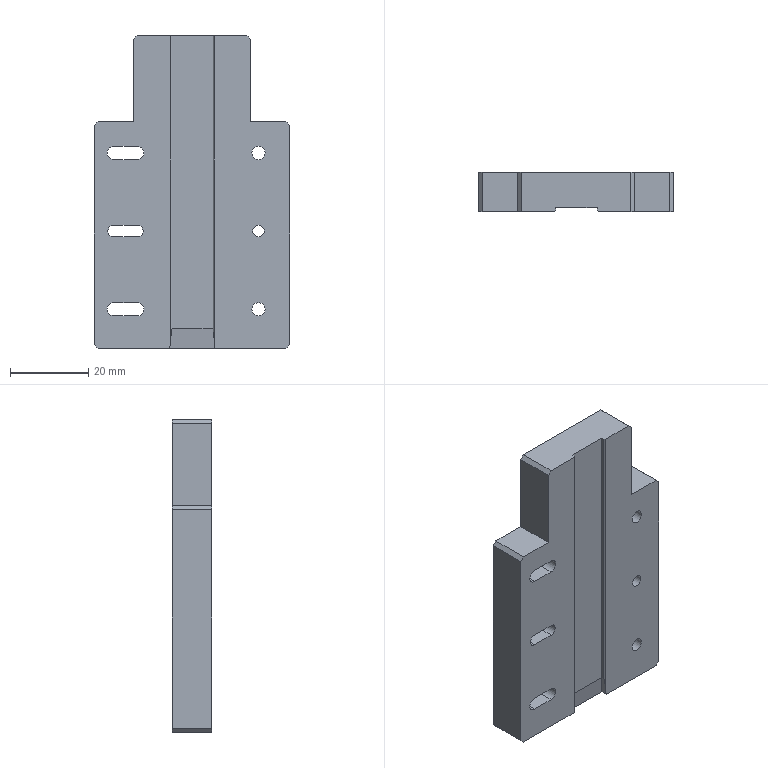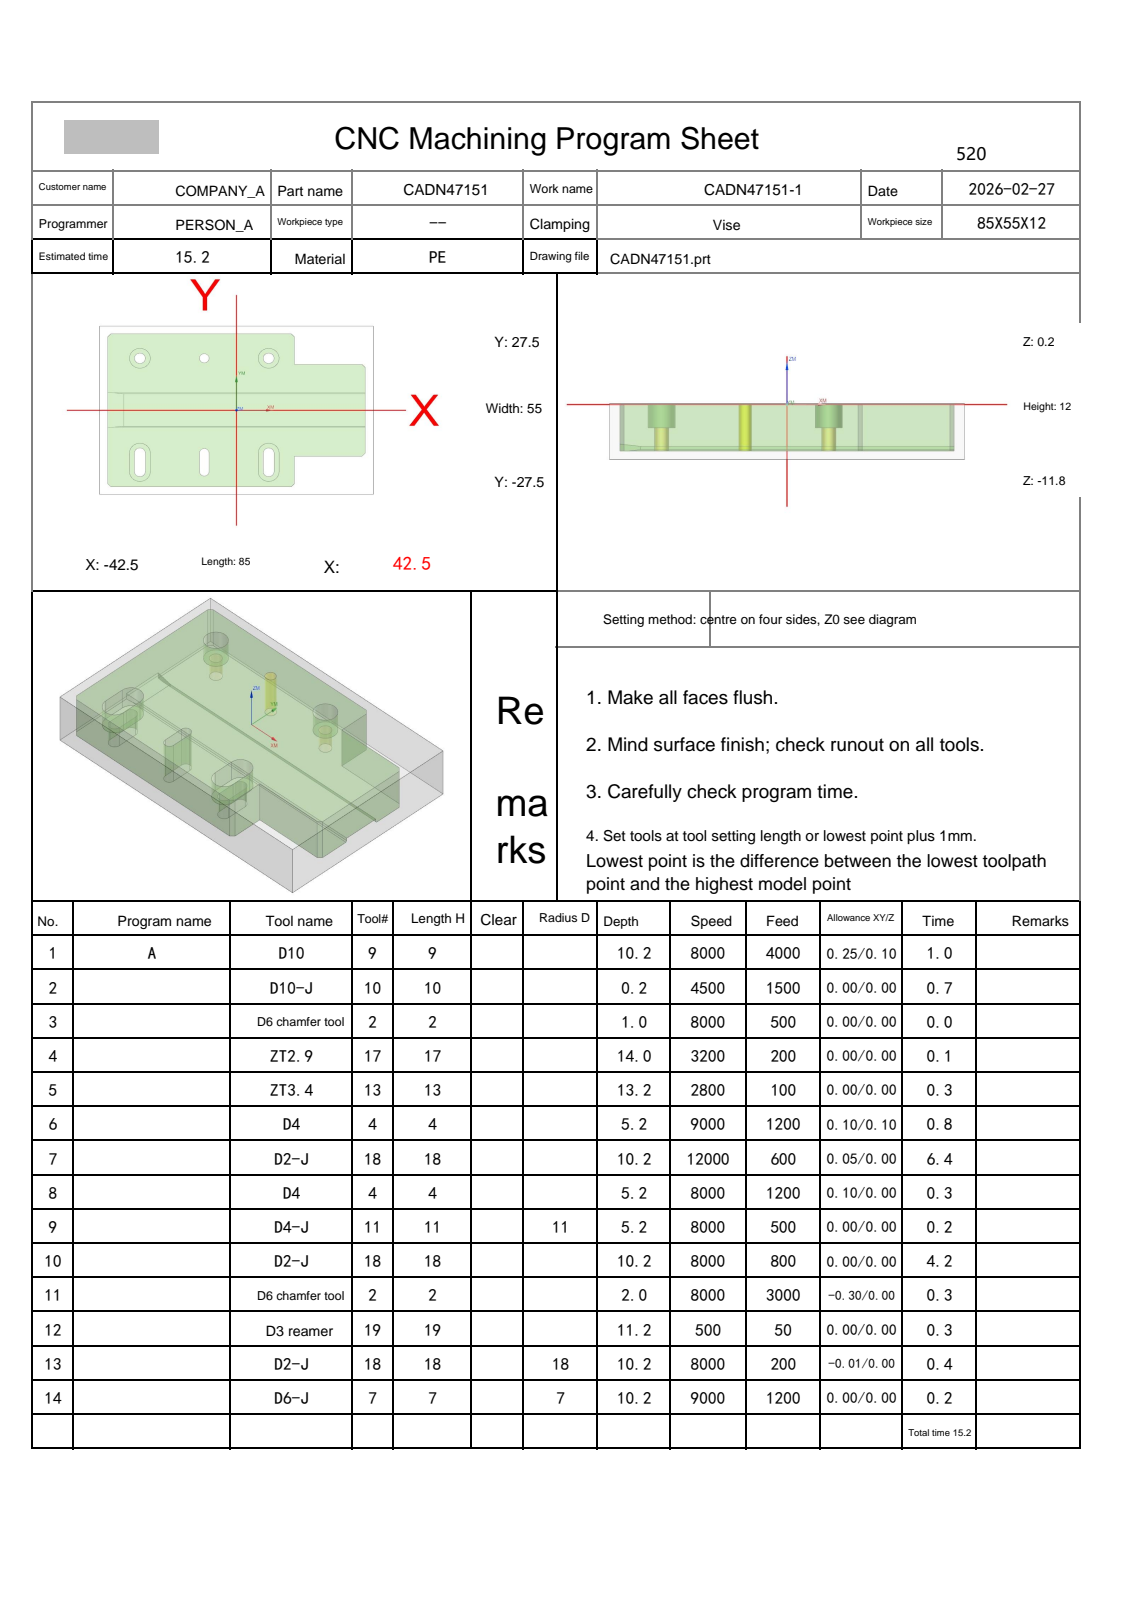NC program | NX | posted by the shop | part box 50 x 10 x 80 mm
Lines 2935 to 4061 of 8100:
N10 T18 M06
(D2-J  D=2. R=0. H=18 ce=0.00 di=0.00)
G00 G90 G54 X19.201 Y20.15 M03 S8000
G43 H18 Z50.
M08
Z.1
G01 X19.199 Y20.149 Z.07 F800.
X19.191 Y20.147 Z.042
X19.18 Y20.144 Z.018
X19.166 Y20.139 Z-.004
X19.149 Y20.133 Z-.023
X19.13 Y20.125 Z-.04
X19.111 Y20.115 Z-.054
X19.091 Y20.103 Z-.066
X19.071 Y20.089 Z-.076
X19.052 Y20.072 Z-.084
X19.035 Y20.053 Z-.09
X19.021 Y20.032 Z-.095
X19.01 Y20.007 Z-.098
X19.003 Y19.98 Z-.099
X19. Y19.95 Z-.1
Y16.
X22.95
X22.964 Y16.014
X22.953 Y16.056 Z-.101
X22.919 Y16.121 Z-.103
X22.864 Y16.209 Z-.104
X22.599 Y16.565 Z-.112
X22.346 Y16.878 Z-.119
X22.146 Y17.111 Z-.125
X21.909 Y17.375 Z-.131
X21.632 Y17.674 Z-.138
X21.322 Y17.995 Z-.146
X20.996 Y18.322 Z-.154
X20.674 Y18.632 Z-.162
X20.376 Y18.909 Z-.169
X20.111 Y19.146 Z-.175
X19.878 Y19.345 Z-.181
X19.566 Y19.599 Z-.188
X19.209 Y19.864 Z-.196
X19.121 Y19.919 Z-.197
X19.056 Y19.953 Z-.199
X19.014 Y19.964 Z-.2
X19. Y19.95
Y16.
X22.95
X22.964 Y16.014
X22.953 Y16.056 Z-.201
X22.919 Y16.121 Z-.203
X22.864 Y16.209 Z-.204
X22.599 Y16.565 Z-.212
X22.346 Y16.878 Z-.219
X22.146 Y17.111 Z-.225
X21.909 Y17.375 Z-.231
X21.632 Y17.674 Z-.238
X21.322 Y17.995 Z-.246
X20.996 Y18.322 Z-.254
X20.674 Y18.632 Z-.262
X20.376 Y18.909 Z-.269
X20.111 Y19.146 Z-.275
X19.878 Y19.345 Z-.281
X19.566 Y19.599 Z-.288
X19.209 Y19.864 Z-.296
X19.121 Y19.919 Z-.297
X19.056 Y19.953 Z-.299
X19.014 Y19.964 Z-.3
X19. Y19.95
Y16.
X22.95
X22.964 Y16.014
X22.953 Y16.056 Z-.301
X22.919 Y16.121 Z-.303
X22.864 Y16.209 Z-.304
X22.599 Y16.565 Z-.312
X22.346 Y16.878 Z-.319
X22.146 Y17.111 Z-.325
X21.909 Y17.375 Z-.331
X21.632 Y17.674 Z-.338
X21.322 Y17.995 Z-.346
X20.996 Y18.322 Z-.354
X20.674 Y18.632 Z-.362
X20.376 Y18.909 Z-.369
X20.111 Y19.146 Z-.375
X19.878 Y19.345 Z-.381
X19.566 Y19.599 Z-.388
X19.209 Y19.864 Z-.396
X19.121 Y19.919 Z-.397
X19.056 Y19.953 Z-.399
X19.014 Y19.964 Z-.4
X19. Y19.95
Y16.
X22.95
X22.964 Y16.014
X22.953 Y16.056 Z-.401
X22.919 Y16.121 Z-.403
X22.864 Y16.209 Z-.404
X22.599 Y16.565 Z-.412
X22.346 Y16.878 Z-.419
X22.146 Y17.111 Z-.425
X21.909 Y17.375 Z-.431
X21.632 Y17.674 Z-.438
X21.322 Y17.995 Z-.446
X20.996 Y18.322 Z-.454
X20.674 Y18.632 Z-.462
X20.376 Y18.909 Z-.469
X20.111 Y19.146 Z-.475
X19.878 Y19.345 Z-.481
X19.566 Y19.599 Z-.488
X19.209 Y19.864 Z-.496
X19.121 Y19.919 Z-.497
X19.056 Y19.953 Z-.499
X19.014 Y19.964 Z-.5
X19. Y19.95
Y16.
X22.95
X22.964 Y16.014
X22.953 Y16.056 Z-.501
X22.919 Y16.121 Z-.503
X22.864 Y16.209 Z-.504
X22.599 Y16.565 Z-.512
X22.346 Y16.878 Z-.519
X22.146 Y17.111 Z-.525
X21.909 Y17.375 Z-.531
X21.632 Y17.674 Z-.538
X21.322 Y17.995 Z-.546
X20.996 Y18.322 Z-.554
X20.674 Y18.632 Z-.562
X20.376 Y18.909 Z-.569
X20.111 Y19.146 Z-.575
X19.878 Y19.345 Z-.581
X19.566 Y19.599 Z-.588
X19.209 Y19.864 Z-.596
X19.121 Y19.919 Z-.597
X19.056 Y19.953 Z-.599
X19.014 Y19.964 Z-.6
X19. Y19.95
Y16.
X22.95
X22.964 Y16.014
X22.953 Y16.056 Z-.601
X22.919 Y16.121 Z-.603
X22.864 Y16.209 Z-.604
X22.599 Y16.565 Z-.612
X22.346 Y16.878 Z-.619
X22.146 Y17.111 Z-.625
X21.909 Y17.375 Z-.631
X21.632 Y17.674 Z-.638
X21.322 Y17.995 Z-.646
X20.996 Y18.322 Z-.654
X20.674 Y18.632 Z-.662
X20.376 Y18.909 Z-.669
X20.111 Y19.146 Z-.675
X19.878 Y19.345 Z-.681
X19.566 Y19.599 Z-.688
X19.209 Y19.864 Z-.696
X19.121 Y19.919 Z-.697
X19.056 Y19.953 Z-.699
X19.014 Y19.964 Z-.7
X19. Y19.95
Y16.
X22.95
X22.964 Y16.014
X22.953 Y16.056 Z-.701
X22.919 Y16.121 Z-.703
X22.864 Y16.209 Z-.704
X22.599 Y16.565 Z-.712
X22.346 Y16.878 Z-.719
X22.146 Y17.111 Z-.725
X21.909 Y17.375 Z-.731
X21.632 Y17.674 Z-.738
X21.322 Y17.995 Z-.746
X20.996 Y18.322 Z-.754
X20.674 Y18.632 Z-.762
X20.376 Y18.909 Z-.769
X20.111 Y19.146 Z-.775
X19.878 Y19.345 Z-.781
X19.566 Y19.599 Z-.788
X19.209 Y19.864 Z-.796
X19.121 Y19.919 Z-.797
X19.056 Y19.953 Z-.799
X19.014 Y19.964 Z-.8
X19. Y19.95
Y16.
X22.95
X22.964 Y16.014
X22.953 Y16.056 Z-.801
X22.919 Y16.121 Z-.803
X22.864 Y16.209 Z-.804
X22.599 Y16.565 Z-.812
X22.346 Y16.878 Z-.819
X22.146 Y17.111 Z-.825
X21.909 Y17.375 Z-.831
X21.632 Y17.674 Z-.838
X21.322 Y17.995 Z-.846
X20.996 Y18.322 Z-.854
X20.674 Y18.632 Z-.862
X20.376 Y18.909 Z-.869
X20.111 Y19.146 Z-.875
X19.878 Y19.345 Z-.881
X19.566 Y19.599 Z-.888
X19.209 Y19.864 Z-.896
X19.121 Y19.919 Z-.897
X19.056 Y19.953 Z-.899
X19.014 Y19.964 Z-.9
X19. Y19.95
Y16.
X22.95
X22.964 Y16.014
X22.953 Y16.056 Z-.901
X22.919 Y16.121 Z-.903
X22.864 Y16.209 Z-.904
X22.599 Y16.565 Z-.912
X22.346 Y16.878 Z-.919
X22.146 Y17.111 Z-.925
X21.909 Y17.375 Z-.931
X21.632 Y17.674 Z-.938
X21.322 Y17.995 Z-.946
X20.996 Y18.322 Z-.954
X20.674 Y18.632 Z-.962
X20.376 Y18.909 Z-.969
X20.111 Y19.146 Z-.975
X19.878 Y19.345 Z-.981
X19.566 Y19.599 Z-.988
X19.209 Y19.864 Z-.996
X19.121 Y19.919 Z-.997
X19.056 Y19.953 Z-.999
X19.014 Y19.964 Z-1.
X19. Y19.95
Y16.
X22.95
X22.964 Y16.014
X22.953 Y16.056 Z-1.001
X22.919 Y16.121 Z-1.003
X22.864 Y16.209 Z-1.004
X22.599 Y16.565 Z-1.012
X22.346 Y16.878 Z-1.019
X22.146 Y17.111 Z-1.025
X21.909 Y17.375 Z-1.031
X21.632 Y17.674 Z-1.038
X21.322 Y17.995 Z-1.046
X20.996 Y18.322 Z-1.054
X20.674 Y18.632 Z-1.062
X20.376 Y18.909 Z-1.069
X20.111 Y19.146 Z-1.075
X19.878 Y19.345 Z-1.081
X19.566 Y19.599 Z-1.088
X19.209 Y19.864 Z-1.096
X19.121 Y19.919 Z-1.097
X19.056 Y19.953 Z-1.099
X19.014 Y19.964 Z-1.1
X19. Y19.95
Y16.
X22.95
X22.964 Y16.014
X22.953 Y16.056 Z-1.101
X22.919 Y16.121 Z-1.103
X22.864 Y16.209 Z-1.104
X22.599 Y16.565 Z-1.112
X22.346 Y16.878 Z-1.119
X22.146 Y17.111 Z-1.125
X21.909 Y17.375 Z-1.131
X21.632 Y17.674 Z-1.138
X21.322 Y17.995 Z-1.146
X20.996 Y18.322 Z-1.154
X20.674 Y18.632 Z-1.162
X20.376 Y18.909 Z-1.169
X20.111 Y19.146 Z-1.175
X19.878 Y19.345 Z-1.181
X19.566 Y19.599 Z-1.188
X19.209 Y19.864 Z-1.196
X19.121 Y19.919 Z-1.197
X19.056 Y19.953 Z-1.199
X19.014 Y19.964 Z-1.2
X19. Y19.95
Y16.
X22.95
X22.964 Y16.014
X22.953 Y16.056 Z-1.201
X22.919 Y16.121 Z-1.203
X22.864 Y16.209 Z-1.204
X22.599 Y16.565 Z-1.212
X22.346 Y16.878 Z-1.219
X22.146 Y17.111 Z-1.225
X21.909 Y17.375 Z-1.231
X21.632 Y17.674 Z-1.238
X21.322 Y17.995 Z-1.246
X20.996 Y18.322 Z-1.254
X20.674 Y18.632 Z-1.262
X20.376 Y18.909 Z-1.269
X20.111 Y19.146 Z-1.275
X19.878 Y19.345 Z-1.281
X19.566 Y19.599 Z-1.288
X19.209 Y19.864 Z-1.296
X19.121 Y19.919 Z-1.297
X19.056 Y19.953 Z-1.299
X19.014 Y19.964 Z-1.3
X19. Y19.95
Y16.
X22.95
X22.964 Y16.014
X22.953 Y16.056 Z-1.301
X22.919 Y16.121 Z-1.303
X22.864 Y16.209 Z-1.304
X22.599 Y16.565 Z-1.312
X22.346 Y16.878 Z-1.319
X22.146 Y17.111 Z-1.325
X21.909 Y17.375 Z-1.331
X21.632 Y17.674 Z-1.338
X21.322 Y17.995 Z-1.346
X20.996 Y18.322 Z-1.354
X20.674 Y18.632 Z-1.362
X20.376 Y18.909 Z-1.369
X20.111 Y19.146 Z-1.375
X19.878 Y19.345 Z-1.381
X19.566 Y19.599 Z-1.388
X19.209 Y19.864 Z-1.396
X19.121 Y19.919 Z-1.397
X19.056 Y19.953 Z-1.399
X19.014 Y19.964 Z-1.4
X19. Y19.95
Y16.
X22.95
X22.964 Y16.014
X22.953 Y16.056 Z-1.401
X22.919 Y16.121 Z-1.403
X22.864 Y16.209 Z-1.404
X22.599 Y16.565 Z-1.412
X22.346 Y16.878 Z-1.419
X22.146 Y17.111 Z-1.425
X21.909 Y17.375 Z-1.431
X21.632 Y17.674 Z-1.438
X21.322 Y17.995 Z-1.446
X20.996 Y18.322 Z-1.454
X20.674 Y18.632 Z-1.462
X20.376 Y18.909 Z-1.469
X20.111 Y19.146 Z-1.475
X19.878 Y19.345 Z-1.481
X19.566 Y19.599 Z-1.488
X19.209 Y19.864 Z-1.496
X19.121 Y19.919 Z-1.497
X19.056 Y19.953 Z-1.499
X19.014 Y19.964 Z-1.5
X19. Y19.95
Y16.
X22.95
X22.964 Y16.014
X22.953 Y16.056 Z-1.501
X22.919 Y16.121 Z-1.503
X22.864 Y16.209 Z-1.504
X22.599 Y16.565 Z-1.512
X22.346 Y16.878 Z-1.519
X22.146 Y17.111 Z-1.525
X21.909 Y17.375 Z-1.531
X21.632 Y17.674 Z-1.538
X21.322 Y17.995 Z-1.546
X20.996 Y18.322 Z-1.554
X20.674 Y18.632 Z-1.562
X20.376 Y18.909 Z-1.569
X20.111 Y19.146 Z-1.575
X19.878 Y19.345 Z-1.581
X19.566 Y19.599 Z-1.588
X19.209 Y19.864 Z-1.596
X19.121 Y19.919 Z-1.597
X19.056 Y19.953 Z-1.599
X19.014 Y19.964 Z-1.6
X19. Y19.95
Y16.
X22.95
X22.964 Y16.014
X22.953 Y16.056 Z-1.601
X22.919 Y16.121 Z-1.603
X22.864 Y16.209 Z-1.604
X22.599 Y16.565 Z-1.612
X22.346 Y16.878 Z-1.619
X22.146 Y17.111 Z-1.625
X21.909 Y17.375 Z-1.631
X21.632 Y17.674 Z-1.638
X21.322 Y17.995 Z-1.646
X20.996 Y18.322 Z-1.654
X20.674 Y18.632 Z-1.662
X20.376 Y18.909 Z-1.669
X20.111 Y19.146 Z-1.675
X19.878 Y19.345 Z-1.681
X19.566 Y19.599 Z-1.688
X19.209 Y19.864 Z-1.696
X19.121 Y19.919 Z-1.697
X19.056 Y19.953 Z-1.699
X19.014 Y19.964 Z-1.7
X19. Y19.95
Y16.
X22.95
X22.964 Y16.014
X22.953 Y16.056 Z-1.701
X22.919 Y16.121 Z-1.703
X22.864 Y16.209 Z-1.704
X22.599 Y16.565 Z-1.712
X22.346 Y16.878 Z-1.719
X22.146 Y17.111 Z-1.725
X21.909 Y17.375 Z-1.731
X21.632 Y17.674 Z-1.738
X21.322 Y17.995 Z-1.746
X20.996 Y18.322 Z-1.754
X20.674 Y18.632 Z-1.762
X20.376 Y18.909 Z-1.769
X20.111 Y19.146 Z-1.775
X19.878 Y19.345 Z-1.781
X19.566 Y19.599 Z-1.788
X19.209 Y19.864 Z-1.796
X19.121 Y19.919 Z-1.797
X19.056 Y19.953 Z-1.799
X19.014 Y19.964 Z-1.8
X19. Y19.95
Y16.
X22.95
X22.964 Y16.014
X22.953 Y16.056 Z-1.801
X22.919 Y16.121 Z-1.803
X22.864 Y16.209 Z-1.804
X22.599 Y16.565 Z-1.812
X22.346 Y16.878 Z-1.819
X22.146 Y17.111 Z-1.825
X21.909 Y17.375 Z-1.831
X21.632 Y17.674 Z-1.838
X21.322 Y17.995 Z-1.846
X20.996 Y18.322 Z-1.854
X20.674 Y18.632 Z-1.862
X20.376 Y18.909 Z-1.869
X20.111 Y19.146 Z-1.875
X19.878 Y19.345 Z-1.881
X19.566 Y19.599 Z-1.888
X19.209 Y19.864 Z-1.896
X19.121 Y19.919 Z-1.897
X19.056 Y19.953 Z-1.899
X19.014 Y19.964 Z-1.9
X19. Y19.95
Y16.
X22.95
X22.964 Y16.014
X22.953 Y16.056 Z-1.901
X22.919 Y16.121 Z-1.903
X22.864 Y16.209 Z-1.904
X22.599 Y16.565 Z-1.912
X22.346 Y16.878 Z-1.919
X22.146 Y17.111 Z-1.925
X21.909 Y17.375 Z-1.931
X21.632 Y17.674 Z-1.938
X21.322 Y17.995 Z-1.946
X20.996 Y18.322 Z-1.954
X20.674 Y18.632 Z-1.962
X20.376 Y18.909 Z-1.969
X20.111 Y19.146 Z-1.975
X19.878 Y19.345 Z-1.981
X19.566 Y19.599 Z-1.988
X19.209 Y19.864 Z-1.996
X19.121 Y19.919 Z-1.997
X19.056 Y19.953 Z-1.999
X19.014 Y19.964 Z-2.
X19. Y19.95
Y16.
X22.95
X22.964 Y16.014
X22.953 Y16.056 Z-2.001
X22.919 Y16.121 Z-2.003
X22.864 Y16.209 Z-2.004
X22.599 Y16.565 Z-2.012
X22.346 Y16.878 Z-2.019
X22.146 Y17.111 Z-2.025
X21.909 Y17.375 Z-2.031
X21.632 Y17.674 Z-2.038
X21.322 Y17.995 Z-2.046
X20.996 Y18.322 Z-2.054
X20.674 Y18.632 Z-2.062
X20.376 Y18.909 Z-2.069
X20.111 Y19.146 Z-2.075
X19.878 Y19.345 Z-2.081
X19.566 Y19.599 Z-2.088
X19.209 Y19.864 Z-2.096
X19.121 Y19.919 Z-2.097
X19.056 Y19.953 Z-2.099
X19.014 Y19.964 Z-2.1
X19. Y19.95
Y16.
X22.95
X22.964 Y16.014
X22.953 Y16.056 Z-2.101
X22.919 Y16.121 Z-2.103
X22.864 Y16.209 Z-2.104
X22.599 Y16.565 Z-2.112
X22.346 Y16.878 Z-2.119
X22.146 Y17.111 Z-2.125
X21.909 Y17.375 Z-2.131
X21.632 Y17.674 Z-2.138
X21.322 Y17.995 Z-2.146
X20.996 Y18.322 Z-2.154
X20.674 Y18.632 Z-2.162
X20.376 Y18.909 Z-2.169
X20.111 Y19.146 Z-2.175
X19.878 Y19.345 Z-2.181
X19.566 Y19.599 Z-2.188
X19.209 Y19.864 Z-2.196
X19.121 Y19.919 Z-2.197
X19.056 Y19.953 Z-2.199
X19.014 Y19.964 Z-2.2
X19. Y19.95
Y16.
X22.95
X22.964 Y16.014
X22.953 Y16.056 Z-2.201
X22.919 Y16.121 Z-2.203
X22.864 Y16.209 Z-2.204
X22.599 Y16.565 Z-2.212
X22.346 Y16.878 Z-2.219
X22.146 Y17.111 Z-2.225
X21.909 Y17.375 Z-2.231
X21.632 Y17.674 Z-2.238
X21.322 Y17.995 Z-2.246
X20.996 Y18.322 Z-2.254
X20.674 Y18.632 Z-2.262
X20.376 Y18.909 Z-2.269
X20.111 Y19.146 Z-2.275
X19.878 Y19.345 Z-2.281
X19.566 Y19.599 Z-2.288
X19.209 Y19.864 Z-2.296
X19.121 Y19.919 Z-2.297
X19.056 Y19.953 Z-2.299
X19.014 Y19.964 Z-2.3
X19. Y19.95
Y16.
X22.95
X22.964 Y16.014
X22.953 Y16.056 Z-2.301
X22.919 Y16.121 Z-2.303
X22.864 Y16.209 Z-2.304
X22.599 Y16.565 Z-2.312
X22.346 Y16.878 Z-2.319
X22.146 Y17.111 Z-2.325
X21.909 Y17.375 Z-2.331
X21.632 Y17.674 Z-2.338
X21.322 Y17.995 Z-2.346
X20.996 Y18.322 Z-2.354
X20.674 Y18.632 Z-2.362
X20.376 Y18.909 Z-2.369
X20.111 Y19.146 Z-2.375
X19.878 Y19.345 Z-2.381
X19.566 Y19.599 Z-2.388
X19.209 Y19.864 Z-2.396
X19.121 Y19.919 Z-2.397
X19.056 Y19.953 Z-2.399
X19.014 Y19.964 Z-2.4
X19. Y19.95
Y16.
X22.95
X22.964 Y16.014
X22.953 Y16.056 Z-2.401
X22.919 Y16.121 Z-2.403
X22.864 Y16.209 Z-2.404
X22.599 Y16.565 Z-2.412
X22.346 Y16.878 Z-2.419
X22.146 Y17.111 Z-2.425
X21.909 Y17.375 Z-2.431
X21.632 Y17.674 Z-2.438
X21.322 Y17.995 Z-2.446
X20.996 Y18.322 Z-2.454
X20.674 Y18.632 Z-2.462
X20.376 Y18.909 Z-2.469
X20.111 Y19.146 Z-2.475
X19.878 Y19.345 Z-2.481
X19.566 Y19.599 Z-2.488
X19.209 Y19.864 Z-2.496
X19.121 Y19.919 Z-2.497
X19.056 Y19.953 Z-2.499
X19.014 Y19.964 Z-2.5
X19. Y19.95
Y16.
X22.95
X22.964 Y16.014
X22.953 Y16.056 Z-2.501
X22.919 Y16.121 Z-2.503
X22.864 Y16.209 Z-2.504
X22.599 Y16.565 Z-2.512
X22.346 Y16.878 Z-2.519
X22.146 Y17.111 Z-2.525
X21.909 Y17.375 Z-2.531
X21.632 Y17.674 Z-2.538
X21.322 Y17.995 Z-2.546
X20.996 Y18.322 Z-2.554
X20.674 Y18.632 Z-2.562
X20.376 Y18.909 Z-2.569
X20.111 Y19.146 Z-2.575
X19.878 Y19.345 Z-2.581
X19.566 Y19.599 Z-2.588
X19.209 Y19.864 Z-2.596
X19.121 Y19.919 Z-2.597
X19.056 Y19.953 Z-2.599
X19.014 Y19.964 Z-2.6
X19. Y19.95
Y16.
X22.95
X22.964 Y16.014
X22.953 Y16.056 Z-2.601
X22.919 Y16.121 Z-2.603
X22.864 Y16.209 Z-2.604
X22.599 Y16.565 Z-2.612
X22.346 Y16.878 Z-2.619
X22.146 Y17.111 Z-2.625
X21.909 Y17.375 Z-2.631
X21.632 Y17.674 Z-2.638
X21.322 Y17.995 Z-2.646
X20.996 Y18.322 Z-2.654
X20.674 Y18.632 Z-2.662
X20.376 Y18.909 Z-2.669
X20.111 Y19.146 Z-2.675
X19.878 Y19.345 Z-2.681
X19.566 Y19.599 Z-2.688
X19.209 Y19.864 Z-2.696
X19.121 Y19.919 Z-2.697
X19.056 Y19.953 Z-2.699
X19.014 Y19.964 Z-2.7
X19. Y19.95
Y16.
X22.95
X22.964 Y16.014
X22.953 Y16.056 Z-2.701
X22.919 Y16.121 Z-2.703
X22.864 Y16.209 Z-2.704
X22.599 Y16.565 Z-2.712
X22.346 Y16.878 Z-2.719
X22.146 Y17.111 Z-2.725
X21.909 Y17.375 Z-2.731
X21.632 Y17.674 Z-2.738
X21.322 Y17.995 Z-2.746
X20.996 Y18.322 Z-2.754
X20.674 Y18.632 Z-2.762
X20.376 Y18.909 Z-2.769
X20.111 Y19.146 Z-2.775
X19.878 Y19.345 Z-2.781
X19.566 Y19.599 Z-2.788
X19.209 Y19.864 Z-2.796
X19.121 Y19.919 Z-2.797
X19.056 Y19.953 Z-2.799
X19.014 Y19.964 Z-2.8
X19. Y19.95
Y16.
X22.95
X22.964 Y16.014
X22.953 Y16.056 Z-2.801
X22.919 Y16.121 Z-2.803
X22.864 Y16.209 Z-2.804
X22.599 Y16.565 Z-2.812
X22.346 Y16.878 Z-2.819
X22.146 Y17.111 Z-2.825
X21.909 Y17.375 Z-2.831
X21.632 Y17.674 Z-2.838
X21.322 Y17.995 Z-2.846
X20.996 Y18.322 Z-2.854
X20.674 Y18.632 Z-2.862
X20.376 Y18.909 Z-2.869
X20.111 Y19.146 Z-2.875
X19.878 Y19.345 Z-2.881
X19.566 Y19.599 Z-2.888
X19.209 Y19.864 Z-2.896
X19.121 Y19.919 Z-2.897
X19.056 Y19.953 Z-2.899
X19.014 Y19.964 Z-2.9
X19. Y19.95
Y16.
X22.95
X22.964 Y16.014
X22.953 Y16.056 Z-2.901
X22.919 Y16.121 Z-2.903
X22.864 Y16.209 Z-2.904
X22.599 Y16.565 Z-2.912
X22.346 Y16.878 Z-2.919
X22.146 Y17.111 Z-2.925
X21.909 Y17.375 Z-2.931
X21.632 Y17.674 Z-2.938
X21.322 Y17.995 Z-2.946
X20.996 Y18.322 Z-2.954
X20.674 Y18.632 Z-2.962
X20.376 Y18.909 Z-2.969
X20.111 Y19.146 Z-2.975
X19.878 Y19.345 Z-2.981
X19.566 Y19.599 Z-2.988
X19.209 Y19.864 Z-2.996
X19.121 Y19.919 Z-2.997
X19.056 Y19.953 Z-2.999
X19.014 Y19.964 Z-3.
X19. Y19.95
Y16.
X22.95
X22.964 Y16.014
X22.953 Y16.056 Z-3.001
X22.919 Y16.121 Z-3.003
X22.864 Y16.209 Z-3.004
X22.599 Y16.565 Z-3.012
X22.346 Y16.878 Z-3.019
X22.146 Y17.111 Z-3.025
X21.909 Y17.375 Z-3.031
X21.632 Y17.674 Z-3.038
X21.322 Y17.995 Z-3.046
X20.996 Y18.322 Z-3.054
X20.674 Y18.632 Z-3.062
X20.376 Y18.909 Z-3.069
X20.111 Y19.146 Z-3.075
X19.878 Y19.345 Z-3.081
X19.566 Y19.599 Z-3.088
X19.209 Y19.864 Z-3.096
X19.121 Y19.919 Z-3.097
X19.056 Y19.953 Z-3.099
X19.014 Y19.964 Z-3.1
X19. Y19.95
Y16.
X22.95
X22.964 Y16.014
X22.953 Y16.056 Z-3.101
X22.919 Y16.121 Z-3.103
X22.864 Y16.209 Z-3.104
X22.599 Y16.565 Z-3.112
X22.346 Y16.878 Z-3.119
X22.146 Y17.111 Z-3.125
X21.909 Y17.375 Z-3.131
X21.632 Y17.674 Z-3.138
X21.322 Y17.995 Z-3.146
X20.996 Y18.322 Z-3.154
X20.674 Y18.632 Z-3.162
X20.376 Y18.909 Z-3.169
X20.111 Y19.146 Z-3.175
X19.878 Y19.345 Z-3.181
X19.566 Y19.599 Z-3.188
X19.209 Y19.864 Z-3.196
X19.121 Y19.919 Z-3.197
X19.056 Y19.953 Z-3.199
X19.014 Y19.964 Z-3.2
X19. Y19.95
Y16.
X22.95
X22.964 Y16.014
X22.953 Y16.056 Z-3.201
X22.919 Y16.121 Z-3.203
X22.864 Y16.209 Z-3.204
X22.599 Y16.565 Z-3.212
X22.346 Y16.878 Z-3.219
X22.146 Y17.111 Z-3.225
X21.909 Y17.375 Z-3.231
X21.632 Y17.674 Z-3.238
X21.322 Y17.995 Z-3.246
X20.996 Y18.322 Z-3.254
X20.674 Y18.632 Z-3.262
X20.376 Y18.909 Z-3.269
X20.111 Y19.146 Z-3.275
X19.878 Y19.345 Z-3.281
X19.566 Y19.599 Z-3.288
X19.209 Y19.864 Z-3.296
X19.121 Y19.919 Z-3.297
X19.056 Y19.953 Z-3.299
X19.014 Y19.964 Z-3.3
X19. Y19.95
Y16.
X22.95
X22.964 Y16.014
X22.953 Y16.056 Z-3.301
X22.919 Y16.121 Z-3.303
X22.864 Y16.209 Z-3.304
X22.599 Y16.565 Z-3.312
X22.346 Y16.878 Z-3.319
X22.146 Y17.111 Z-3.325
X21.909 Y17.375 Z-3.331
X21.632 Y17.674 Z-3.338
X21.322 Y17.995 Z-3.346
X20.996 Y18.322 Z-3.354
X20.674 Y18.632 Z-3.362
X20.376 Y18.909 Z-3.369
X20.111 Y19.146 Z-3.375
X19.878 Y19.345 Z-3.381
X19.566 Y19.599 Z-3.388
X19.209 Y19.864 Z-3.396
X19.121 Y19.919 Z-3.397
X19.056 Y19.953 Z-3.399
X19.014 Y19.964 Z-3.4
X19. Y19.95
Y16.
X22.95
X22.964 Y16.014
X22.953 Y16.056 Z-3.401
X22.919 Y16.121 Z-3.403
X22.864 Y16.209 Z-3.404
X22.599 Y16.565 Z-3.412
X22.346 Y16.878 Z-3.419
X22.146 Y17.111 Z-3.425
X21.909 Y17.375 Z-3.431
X21.632 Y17.674 Z-3.438
X21.322 Y17.995 Z-3.446
X20.996 Y18.322 Z-3.454
X20.674 Y18.632 Z-3.462
X20.376 Y18.909 Z-3.469
X20.111 Y19.146 Z-3.475
X19.878 Y19.345 Z-3.481
X19.566 Y19.599 Z-3.488
X19.209 Y19.864 Z-3.496
X19.121 Y19.919 Z-3.497
X19.056 Y19.953 Z-3.499
X19.014 Y19.964 Z-3.5
X19. Y19.95
Y16.
X22.95
X22.964 Y16.014
X22.953 Y16.056 Z-3.501
X22.919 Y16.121 Z-3.503
X22.864 Y16.209 Z-3.504
X22.599 Y16.565 Z-3.512
X22.346 Y16.878 Z-3.519
X22.146 Y17.111 Z-3.525
X21.909 Y17.375 Z-3.531
X21.632 Y17.674 Z-3.538
X21.322 Y17.995 Z-3.546
X20.996 Y18.322 Z-3.554
X20.674 Y18.632 Z-3.562
X20.376 Y18.909 Z-3.569
X20.111 Y19.146 Z-3.575
X19.878 Y19.345 Z-3.581
X19.566 Y19.599 Z-3.588
X19.209 Y19.864 Z-3.596
X19.121 Y19.919 Z-3.597
X19.056 Y19.953 Z-3.599
X19.014 Y19.964 Z-3.6
X19. Y19.95
Y16.
X22.95
X22.964 Y16.014
X22.953 Y16.056 Z-3.601
X22.919 Y16.121 Z-3.603
X22.864 Y16.209 Z-3.604
X22.599 Y16.565 Z-3.612
X22.346 Y16.878 Z-3.619
X22.146 Y17.111 Z-3.625
X21.909 Y17.375 Z-3.631
X21.632 Y17.674 Z-3.638
X21.322 Y17.995 Z-3.646
X20.996 Y18.322 Z-3.654
X20.674 Y18.632 Z-3.662
X20.376 Y18.909 Z-3.669
X20.111 Y19.146 Z-3.675
X19.878 Y19.345 Z-3.681
X19.566 Y19.599 Z-3.688
X19.209 Y19.864 Z-3.696
X19.121 Y19.919 Z-3.697
X19.056 Y19.953 Z-3.699
X19.014 Y19.964 Z-3.7
X19. Y19.95
Y16.
X22.95
X22.964 Y16.014
X22.953 Y16.056 Z-3.701
X22.919 Y16.121 Z-3.703
X22.864 Y16.209 Z-3.704
X22.599 Y16.565 Z-3.712
X22.346 Y16.878 Z-3.719
X22.146 Y17.111 Z-3.725
X21.909 Y17.375 Z-3.731
X21.632 Y17.674 Z-3.738
X21.322 Y17.995 Z-3.746
X20.996 Y18.322 Z-3.754
X20.674 Y18.632 Z-3.762
X20.376 Y18.909 Z-3.769
X20.111 Y19.146 Z-3.775
X19.878 Y19.345 Z-3.781
X19.566 Y19.599 Z-3.788
X19.209 Y19.864 Z-3.796
X19.121 Y19.919 Z-3.797
X19.056 Y19.953 Z-3.799
X19.014 Y19.964 Z-3.8
X19. Y19.95
Y16.
X22.95
X22.964 Y16.014
X22.953 Y16.056 Z-3.801
X22.919 Y16.121 Z-3.803
X22.864 Y16.209 Z-3.804
X22.599 Y16.565 Z-3.812
X22.346 Y16.878 Z-3.819
X22.146 Y17.111 Z-3.825
X21.909 Y17.375 Z-3.831
X21.632 Y17.674 Z-3.838
X21.322 Y17.995 Z-3.846
X20.996 Y18.322 Z-3.854
X20.674 Y18.632 Z-3.862
X20.376 Y18.909 Z-3.869
X20.111 Y19.146 Z-3.875
X19.878 Y19.345 Z-3.881
X19.566 Y19.599 Z-3.888
X19.209 Y19.864 Z-3.896
X19.121 Y19.919 Z-3.897
X19.056 Y19.953 Z-3.899
X19.014 Y19.964 Z-3.9
X19. Y19.95
Y16.
X22.95
X22.964 Y16.014
X22.953 Y16.056 Z-3.901
X22.919 Y16.121 Z-3.903
X22.864 Y16.209 Z-3.904
X22.599 Y16.565 Z-3.912
X22.346 Y16.878 Z-3.919
X22.146 Y17.111 Z-3.925
X21.909 Y17.375 Z-3.931
X21.632 Y17.674 Z-3.938
X21.322 Y17.995 Z-3.946
X20.996 Y18.322 Z-3.954
X20.674 Y18.632 Z-3.962
X20.376 Y18.909 Z-3.969
X20.111 Y19.146 Z-3.975
X19.878 Y19.345 Z-3.981
X19.566 Y19.599 Z-3.988
X19.209 Y19.864 Z-3.996
X19.121 Y19.919 Z-3.997
X19.056 Y19.953 Z-3.999
X19.014 Y19.964 Z-4.
X19. Y19.95
Y16.
X22.95
X22.964 Y16.014
X22.953 Y16.056 Z-4.001
X22.919 Y16.121 Z-4.003
X22.864 Y16.209 Z-4.004
X22.599 Y16.565 Z-4.012
X22.346 Y16.878 Z-4.019
X22.146 Y17.111 Z-4.025
X21.909 Y17.375 Z-4.031
X21.632 Y17.674 Z-4.038
X21.322 Y17.995 Z-4.046
X20.996 Y18.322 Z-4.054
X20.674 Y18.632 Z-4.062
X20.376 Y18.909 Z-4.069
X20.111 Y19.146 Z-4.075
X19.878 Y19.345 Z-4.081
X19.566 Y19.599 Z-4.088
X19.209 Y19.864 Z-4.096
X19.121 Y19.919 Z-4.097
X19.056 Y19.953 Z-4.099
X19.014 Y19.964 Z-4.1
X19. Y19.95
Y16.
X22.95
X22.964 Y16.014
X22.953 Y16.056 Z-4.101
X22.919 Y16.121 Z-4.103
X22.864 Y16.209 Z-4.104
X22.599 Y16.565 Z-4.112
X22.346 Y16.878 Z-4.119
X22.146 Y17.111 Z-4.125
X21.909 Y17.375 Z-4.131
X21.632 Y17.674 Z-4.138
X21.322 Y17.995 Z-4.146
X20.996 Y18.322 Z-4.154
X20.674 Y18.632 Z-4.162
X20.376 Y18.909 Z-4.169
X20.111 Y19.146 Z-4.175
X19.878 Y19.345 Z-4.181
X19.566 Y19.599 Z-4.188
X19.209 Y19.864 Z-4.196
X19.121 Y19.919 Z-4.197
X19.056 Y19.953 Z-4.199
X19.014 Y19.964 Z-4.2
X19. Y19.95
Y16.
X22.95
X22.964 Y16.014
X22.953 Y16.056 Z-4.201
X22.919 Y16.121 Z-4.203
X22.864 Y16.209 Z-4.204
X22.599 Y16.565 Z-4.212
X22.346 Y16.878 Z-4.219
X22.146 Y17.111 Z-4.225
X21.909 Y17.375 Z-4.231
X21.632 Y17.674 Z-4.238
X21.322 Y17.995 Z-4.246
X20.996 Y18.322 Z-4.254
X20.674 Y18.632 Z-4.262
X20.376 Y18.909 Z-4.269
X20.111 Y19.146 Z-4.275
X19.878 Y19.345 Z-4.281
X19.566 Y19.599 Z-4.288
X19.209 Y19.864 Z-4.296
X19.121 Y19.919 Z-4.297
X19.056 Y19.953 Z-4.299
X19.014 Y19.964 Z-4.3
X19. Y19.95
Y16.
X22.95
X22.964 Y16.014
X22.953 Y16.056 Z-4.301
X22.919 Y16.121 Z-4.303
X22.864 Y16.209 Z-4.304
X22.599 Y16.565 Z-4.312
X22.346 Y16.878 Z-4.319
X22.146 Y17.111 Z-4.325
X21.909 Y17.375 Z-4.331
X21.632 Y17.674 Z-4.338
X21.322 Y17.995 Z-4.346
X20.996 Y18.322 Z-4.354
X20.674 Y18.632 Z-4.362
X20.376 Y18.909 Z-4.369
X20.111 Y19.146 Z-4.375
X19.878 Y19.345 Z-4.381
X19.566 Y19.599 Z-4.388
X19.209 Y19.864 Z-4.396
X19.121 Y19.919 Z-4.397
X19.056 Y19.953 Z-4.399
X19.014 Y19.964 Z-4.4
X19. Y19.95
Y16.
X22.95
X22.964 Y16.014
X22.953 Y16.056 Z-4.401
X22.919 Y16.121 Z-4.403
X22.864 Y16.209 Z-4.404
X22.599 Y16.565 Z-4.412
X22.346 Y16.878 Z-4.419
X22.146 Y17.111 Z-4.425
X21.909 Y17.375 Z-4.431
X21.632 Y17.674 Z-4.438
X21.322 Y17.995 Z-4.446
X20.996 Y18.322 Z-4.454
X20.674 Y18.632 Z-4.462
X20.376 Y18.909 Z-4.469
X20.111 Y19.146 Z-4.475
X19.878 Y19.345 Z-4.481
X19.566 Y19.599 Z-4.488
X19.209 Y19.864 Z-4.496
X19.121 Y19.919 Z-4.497
X19.056 Y19.953 Z-4.499
X19.014 Y19.964 Z-4.5
X19. Y19.95
Y16.
X22.95
X22.964 Y16.014
X22.953 Y16.056 Z-4.501
X22.919 Y16.121 Z-4.503
X22.864 Y16.209 Z-4.504
X22.599 Y16.565 Z-4.512
X22.346 Y16.878 Z-4.519
X22.146 Y17.111 Z-4.525
X21.909 Y17.375 Z-4.531
X21.632 Y17.674 Z-4.538
X21.322 Y17.995 Z-4.546
X20.996 Y18.322 Z-4.554
X20.674 Y18.632 Z-4.562
X20.376 Y18.909 Z-4.569
X20.111 Y19.146 Z-4.575
X19.878 Y19.345 Z-4.581
X19.566 Y19.599 Z-4.588
X19.209 Y19.864 Z-4.596
X19.121 Y19.919 Z-4.597
X19.056 Y19.953 Z-4.599
X19.014 Y19.964 Z-4.6
X19. Y19.95
Y16.
X22.95
X22.964 Y16.014
X22.953 Y16.056 Z-4.601
X22.919 Y16.121 Z-4.603
X22.864 Y16.209 Z-4.604
X22.599 Y16.565 Z-4.612
X22.346 Y16.878 Z-4.619
X22.146 Y17.111 Z-4.625
X21.909 Y17.375 Z-4.631
X21.632 Y17.674 Z-4.638
X21.322 Y17.995 Z-4.646
X20.996 Y18.322 Z-4.654
X20.674 Y18.632 Z-4.662
X20.376 Y18.909 Z-4.669
X20.111 Y19.146 Z-4.675
X19.878 Y19.345 Z-4.681
X19.566 Y19.599 Z-4.688
X19.209 Y19.864 Z-4.696
X19.121 Y19.919 Z-4.697
X19.056 Y19.953 Z-4.699
X19.014 Y19.964 Z-4.7
X19. Y19.95
Y16.
X22.95
X22.964 Y16.014
X22.953 Y16.056 Z-4.701
X22.919 Y16.121 Z-4.703
X22.864 Y16.209 Z-4.704
X22.599 Y16.565 Z-4.712
X22.346 Y16.878 Z-4.719
X22.146 Y17.111 Z-4.725
X21.909 Y17.375 Z-4.731
X21.632 Y17.674 Z-4.738
X21.322 Y17.995 Z-4.746
X20.996 Y18.322 Z-4.754
X20.674 Y18.632 Z-4.762
X20.376 Y18.909 Z-4.769
X20.111 Y19.146 Z-4.775
X19.878 Y19.345 Z-4.781
X19.566 Y19.599 Z-4.788
X19.209 Y19.864 Z-4.796
X19.121 Y19.919 Z-4.797
X19.056 Y19.953 Z-4.799
X19.014 Y19.964 Z-4.8
X19. Y19.95
Y16.
X22.95
X22.964 Y16.014
X22.953 Y16.056 Z-4.801
X22.919 Y16.121 Z-4.803
X22.864 Y16.209 Z-4.804
X22.599 Y16.565 Z-4.812
X22.346 Y16.878 Z-4.819
X22.146 Y17.111 Z-4.825
X21.909 Y17.375 Z-4.831
X21.632 Y17.674 Z-4.838
X21.322 Y17.995 Z-4.846
X20.996 Y18.322 Z-4.854
X20.674 Y18.632 Z-4.862
X20.376 Y18.909 Z-4.869
X20.111 Y19.146 Z-4.875
X19.878 Y19.345 Z-4.881
X19.566 Y19.599 Z-4.888
X19.209 Y19.864 Z-4.896
X19.121 Y19.919 Z-4.897
X19.056 Y19.953 Z-4.899
X19.014 Y19.964 Z-4.9
X19. Y19.95
Y16.
X22.95